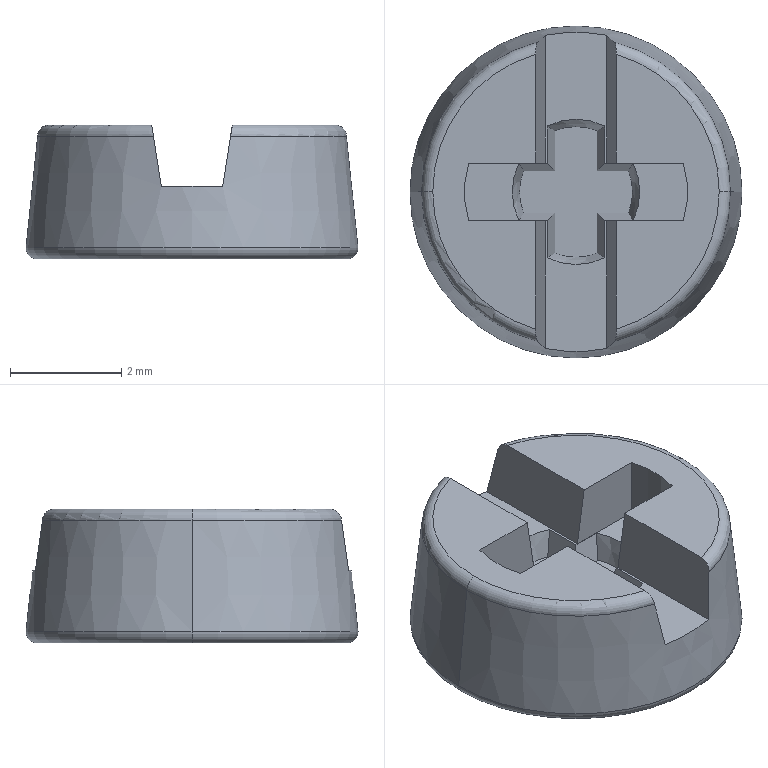Part | STEP file | 2023_07_21_12_39_19_0137 | 1 solid | 35 faces | box 5.956 x 5.956 x 2.4 mm | volume 49.622 mm3 | plane 21 | torus 6 | cone 6 | cylinder 2 | commonest cylinder face diameters 3.7 x2
STEP:
#1=CARTESIAN_POINT('',(12.522,55.,30.7));
#2=VERTEX_POINT('',#1);
#3=CARTESIAN_POINT('',(18.478,55.,30.7));
#4=VERTEX_POINT('',#3);
#5=CARTESIAN_POINT('',(15.5,55.,30.7));
#6=DIRECTION('',(0.,0.,-1.));
#7=DIRECTION('',(-1.,0.,0.));
#8=AXIS2_PLACEMENT_3D('',#5,#6,#7);
#9=CIRCLE('',#8,2.978);
#10=EDGE_CURVE('',#2,#4,#9,.T.);
#11=ORIENTED_EDGE('',*,*,#10,.T.);
#12=CARTESIAN_POINT('',(18.278,55.,30.5));
#13=VERTEX_POINT('',#12);
#14=CARTESIAN_POINT('',(18.278,55.,30.7));
#15=DIRECTION('',(0.,1.,0.));
#16=DIRECTION('',(-1.,0.,0.));
#17=AXIS2_PLACEMENT_3D('',#14,#15,#16);
#18=CIRCLE('',#17,0.2);
#19=EDGE_CURVE('',#4,#13,#18,.T.);
#20=ORIENTED_EDGE('',*,*,#19,.T.);
#21=CARTESIAN_POINT('',(12.722,55.,30.5));
#22=VERTEX_POINT('',#21);
#23=CARTESIAN_POINT('',(15.5,55.,30.5));
#24=DIRECTION('',(0.,0.,-1.));
#25=DIRECTION('',(-1.,0.,0.));
#26=AXIS2_PLACEMENT_3D('',#23,#24,#25);
#27=CIRCLE('',#26,2.778);
#28=EDGE_CURVE('',#22,#13,#27,.T.);
#29=ORIENTED_EDGE('',*,*,#28,.F.);
#30=CARTESIAN_POINT('',(12.722,55.,30.7));
#31=DIRECTION('',(0.,-1.,0.));
#32=DIRECTION('',(0.,0.,-1.));
#33=AXIS2_PLACEMENT_3D('',#30,#31,#32);
#34=CIRCLE('',#33,0.2);
#35=EDGE_CURVE('',#2,#22,#34,.T.);
#36=ORIENTED_EDGE('',*,*,#35,.F.);
#37=EDGE_LOOP('',(#11,#20,#29,#36));
#38=FACE_OUTER_BOUND('',#37,.T.);
#39=CARTESIAN_POINT('',(15.5,55.,30.7));
#40=DIRECTION('',(0.,0.,-1.));
#41=DIRECTION('',(-1.,0.,0.));
#42=AXIS2_PLACEMENT_3D('',#39,#40,#41);
#43=TOROIDAL_SURFACE('',#42,2.778,0.2);
#44=ADVANCED_FACE('',(#38),#43,.T.);
#45=CARTESIAN_POINT('',(16.192,57.682,32.7));
#46=VERTEX_POINT('',#45);
#47=CARTESIAN_POINT('',(18.27,55.,32.7));
#48=VERTEX_POINT('',#47);
#49=CARTESIAN_POINT('',(15.5,55.,32.7));
#50=DIRECTION('',(0.,0.,-1.));
#51=DIRECTION('',(-1.,0.,0.));
#52=AXIS2_PLACEMENT_3D('',#49,#50,#51);
#53=CIRCLE('',#52,2.77);
#54=EDGE_CURVE('',#46,#48,#53,.T.);
#55=ORIENTED_EDGE('',*,*,#54,.T.);
#56=CARTESIAN_POINT('',(18.374,55.,31.7));
#57=DIRECTION('',(0.1036,0.,-0.9946));
#58=VECTOR('',#57,1000.);
#59=LINE('',#56,#58);
#60=EDGE_CURVE('',#48,#4,#59,.T.);
#61=ORIENTED_EDGE('',*,*,#60,.T.);
#62=ORIENTED_EDGE('',*,*,#10,.F.);
#63=CARTESIAN_POINT('',(12.73,55.,32.7));
#64=VERTEX_POINT('',#63);
#65=CARTESIAN_POINT('',(12.626,55.,31.7));
#66=DIRECTION('',(-0.1036,0.,-0.9946));
#67=VECTOR('',#66,1000.);
#68=LINE('',#65,#67);
#69=EDGE_CURVE('',#64,#2,#68,.T.);
#70=ORIENTED_EDGE('',*,*,#69,.F.);
#71=CARTESIAN_POINT('',(14.808,57.682,32.7));
#72=VERTEX_POINT('',#71);
#73=CARTESIAN_POINT('',(15.5,55.,32.7));
#74=DIRECTION('',(0.,0.,-1.));
#75=DIRECTION('',(-1.,0.,0.));
#76=AXIS2_PLACEMENT_3D('',#73,#74,#75);
#77=CIRCLE('',#76,2.77);
#78=EDGE_CURVE('',#64,#72,#77,.T.);
#79=ORIENTED_EDGE('',*,*,#78,.T.);
#80=CARTESIAN_POINT('',(14.95,57.81,31.8));
#81=VERTEX_POINT('',#80);
#82=CARTESIAN_POINT('',(14.808,57.682,32.7));
#83=CARTESIAN_POINT('',(14.854,57.725,32.407));
#84=CARTESIAN_POINT('',(14.902,57.768,32.107));
#85=CARTESIAN_POINT('',(14.95,57.81,31.8));
#86=(BOUNDED_CURVE()B_SPLINE_CURVE(3,(#82,#83,#84,#85),.UNSPECIFIED.,.F.,.F.)B_SPLINE_CURVE_WITH_KNOTS((4,4),(3.815,3.854),.UNSPECIFIED.)CURVE()GEOMETRIC_REPRESENTATION_ITEM()RATIONAL_B_SPLINE_CURVE((1.,0.9999,0.9999,1.))REPRESENTATION_ITEM(''));
#87=EDGE_CURVE('',#72,#81,#86,.T.);
#88=ORIENTED_EDGE('',*,*,#87,.T.);
#89=CARTESIAN_POINT('',(16.05,57.81,31.8));
#90=VERTEX_POINT('',#89);
#91=CARTESIAN_POINT('',(15.5,55.,31.8));
#92=DIRECTION('',(0.,0.,-1.));
#93=DIRECTION('',(-1.,0.,0.));
#94=AXIS2_PLACEMENT_3D('',#91,#92,#93);
#95=CIRCLE('',#94,2.864);
#96=EDGE_CURVE('',#81,#90,#95,.T.);
#97=ORIENTED_EDGE('',*,*,#96,.T.);
#98=CARTESIAN_POINT('',(16.05,57.81,31.8));
#99=CARTESIAN_POINT('',(16.098,57.768,32.107));
#100=CARTESIAN_POINT('',(16.146,57.725,32.407));
#101=CARTESIAN_POINT('',(16.192,57.682,32.7));
#102=(BOUNDED_CURVE()B_SPLINE_CURVE(3,(#98,#99,#100,#101),.UNSPECIFIED.,.F.,.F.)B_SPLINE_CURVE_WITH_KNOTS((4,4),(5.571,5.61),.UNSPECIFIED.)CURVE()GEOMETRIC_REPRESENTATION_ITEM()RATIONAL_B_SPLINE_CURVE((1.,0.9999,0.9999,1.))REPRESENTATION_ITEM(''));
#103=EDGE_CURVE('',#90,#46,#102,.T.);
#104=ORIENTED_EDGE('',*,*,#103,.T.);
#105=EDGE_LOOP('',(#55,#61,#62,#70,#79,#88,#97,#104));
#106=FACE_OUTER_BOUND('',#105,.T.);
#107=CARTESIAN_POINT('',(15.5,55.,31.7));
#108=DIRECTION('',(0.,0.,-1.));
#109=DIRECTION('',(-1.,0.,0.));
#110=AXIS2_PLACEMENT_3D('',#107,#108,#109);
#111=CONICAL_SURFACE('',#110,2.874,0.1038);
#112=ADVANCED_FACE('',(#106),#111,.T.);
#113=CARTESIAN_POINT('',(14.777,52.534,32.9));
#114=VERTEX_POINT('',#113);
#115=CARTESIAN_POINT('',(12.93,55.,32.9));
#116=VERTEX_POINT('',#115);
#117=CARTESIAN_POINT('',(15.5,55.,32.9));
#118=DIRECTION('',(0.,0.,-1.));
#119=DIRECTION('',(-1.,0.,0.));
#120=AXIS2_PLACEMENT_3D('',#117,#118,#119);
#121=CIRCLE('',#120,2.57);
#122=EDGE_CURVE('',#114,#116,#121,.T.);
#123=ORIENTED_EDGE('',*,*,#122,.T.);
#124=CARTESIAN_POINT('',(12.93,55.,32.7));
#125=DIRECTION('',(0.,-1.,0.));
#126=DIRECTION('',(0.,0.,-1.));
#127=AXIS2_PLACEMENT_3D('',#124,#125,#126);
#128=CIRCLE('',#127,0.2);
#129=EDGE_CURVE('',#116,#64,#128,.T.);
#130=ORIENTED_EDGE('',*,*,#129,.T.);
#131=CARTESIAN_POINT('',(14.808,52.318,32.7));
#132=VERTEX_POINT('',#131);
#133=CARTESIAN_POINT('',(15.5,55.,32.7));
#134=DIRECTION('',(0.,0.,-1.));
#135=DIRECTION('',(-1.,0.,0.));
#136=AXIS2_PLACEMENT_3D('',#133,#134,#135);
#137=CIRCLE('',#136,2.77);
#138=EDGE_CURVE('',#132,#64,#137,.T.);
#139=ORIENTED_EDGE('',*,*,#138,.F.);
#140=CARTESIAN_POINT('',(14.808,52.318,32.7));
#141=CARTESIAN_POINT('',(14.804,52.319,32.723));
#142=CARTESIAN_POINT('',(14.8,52.324,32.748));
#143=CARTESIAN_POINT('',(14.795,52.341,32.785));
#144=CARTESIAN_POINT('',(14.793,52.347,32.797));
#145=CARTESIAN_POINT('',(14.79,52.36,32.815));
#146=CARTESIAN_POINT('',(14.789,52.367,32.823));
#147=CARTESIAN_POINT('',(14.787,52.375,32.832));
#148=CARTESIAN_POINT('',(14.787,52.38,32.837));
#149=CARTESIAN_POINT('',(14.786,52.384,32.841));
#150=CARTESIAN_POINT('',(14.784,52.4,32.855));
#151=CARTESIAN_POINT('',(14.781,52.42,32.871));
#152=CARTESIAN_POINT('',(14.777,52.489,32.898));
#153=CARTESIAN_POINT('',(14.777,52.517,32.9));
#154=CARTESIAN_POINT('',(14.777,52.534,32.9));
#155=B_SPLINE_CURVE_WITH_KNOTS('',3,(#140,#141,#142,#143,#144,#145,#146,#147,#148,#149,#150,#151,#152,#153,#154),.UNSPECIFIED.,.F.,.F.,(4,2,2,1,2,2,2,4),(0.,0.25,0.375,0.4375,0.4688,0.5,0.75,1.),.UNSPECIFIED.);
#156=EDGE_CURVE('',#132,#114,#155,.T.);
#157=ORIENTED_EDGE('',*,*,#156,.T.);
#158=EDGE_LOOP('',(#123,#130,#139,#157));
#159=FACE_OUTER_BOUND('',#158,.T.);
#160=CARTESIAN_POINT('',(15.5,55.,32.7));
#161=DIRECTION('',(0.,0.,-1.));
#162=DIRECTION('',(-1.,0.,0.));
#163=AXIS2_PLACEMENT_3D('',#160,#161,#162);
#164=TOROIDAL_SURFACE('',#163,2.57,0.2);
#165=ADVANCED_FACE('',(#159),#164,.T.);
#166=CARTESIAN_POINT('',(16.223,57.466,32.9));
#167=VERTEX_POINT('',#166);
#168=CARTESIAN_POINT('',(18.07,55.,32.9));
#169=VERTEX_POINT('',#168);
#170=CARTESIAN_POINT('',(15.5,55.,32.9));
#171=DIRECTION('',(0.,0.,-1.));
#172=DIRECTION('',(-1.,0.,0.));
#173=AXIS2_PLACEMENT_3D('',#170,#171,#172);
#174=CIRCLE('',#173,2.57);
#175=EDGE_CURVE('',#167,#169,#174,.T.);
#176=ORIENTED_EDGE('',*,*,#175,.T.);
#177=CARTESIAN_POINT('',(18.07,55.,32.7));
#178=DIRECTION('',(0.,1.,0.));
#179=DIRECTION('',(0.,0.,1.));
#180=AXIS2_PLACEMENT_3D('',#177,#178,#179);
#181=CIRCLE('',#180,0.2);
#182=EDGE_CURVE('',#169,#48,#181,.T.);
#183=ORIENTED_EDGE('',*,*,#182,.T.);
#184=ORIENTED_EDGE('',*,*,#54,.F.);
#185=CARTESIAN_POINT('',(16.192,57.682,32.7));
#186=CARTESIAN_POINT('',(16.196,57.681,32.723));
#187=CARTESIAN_POINT('',(16.2,57.676,32.748));
#188=CARTESIAN_POINT('',(16.205,57.659,32.785));
#189=CARTESIAN_POINT('',(16.207,57.653,32.797));
#190=CARTESIAN_POINT('',(16.21,57.64,32.815));
#191=CARTESIAN_POINT('',(16.211,57.633,32.823));
#192=CARTESIAN_POINT('',(16.213,57.625,32.832));
#193=CARTESIAN_POINT('',(16.213,57.62,32.837));
#194=CARTESIAN_POINT('',(16.214,57.616,32.841));
#195=CARTESIAN_POINT('',(16.216,57.6,32.855));
#196=CARTESIAN_POINT('',(16.219,57.58,32.871));
#197=CARTESIAN_POINT('',(16.223,57.511,32.898));
#198=CARTESIAN_POINT('',(16.223,57.483,32.9));
#199=CARTESIAN_POINT('',(16.223,57.466,32.9));
#200=B_SPLINE_CURVE_WITH_KNOTS('',3,(#185,#186,#187,#188,#189,#190,#191,#192,#193,#194,#195,#196,#197,#198,#199),.UNSPECIFIED.,.F.,.F.,(4,2,2,1,2,2,2,4),(0.,0.25,0.375,0.4375,0.4688,0.5,0.75,1.),.UNSPECIFIED.);
#201=EDGE_CURVE('',#46,#167,#200,.T.);
#202=ORIENTED_EDGE('',*,*,#201,.T.);
#203=EDGE_LOOP('',(#176,#183,#184,#202));
#204=FACE_OUTER_BOUND('',#203,.T.);
#205=CARTESIAN_POINT('',(15.5,55.,32.7));
#206=DIRECTION('',(0.,0.,-1.));
#207=DIRECTION('',(1.,0.,0.));
#208=AXIS2_PLACEMENT_3D('',#205,#206,#207);
#209=TOROIDAL_SURFACE('',#208,2.57,0.2);
#210=ADVANCED_FACE('',(#204),#209,.T.);
#211=ORIENTED_EDGE('',*,*,#28,.T.);
#212=CARTESIAN_POINT('',(15.5,55.,30.5));
#213=DIRECTION('',(0.,0.,-1.));
#214=DIRECTION('',(-1.,0.,0.));
#215=AXIS2_PLACEMENT_3D('',#212,#213,#214);
#216=CIRCLE('',#215,2.778);
#217=EDGE_CURVE('',#13,#22,#216,.T.);
#218=ORIENTED_EDGE('',*,*,#217,.T.);
#219=EDGE_LOOP('',(#211,#218));
#220=FACE_OUTER_BOUND('',#219,.T.);
#221=CARTESIAN_POINT('',(14.111,55.,30.5));
#222=DIRECTION('',(0.,0.,-1.));
#223=DIRECTION('',(-1.,0.,0.));
#224=AXIS2_PLACEMENT_3D('',#221,#222,#223);
#225=PLANE('',#224);
#226=ADVANCED_FACE('',(#220),#225,.T.);
#227=CARTESIAN_POINT('',(17.427,54.485,32.9));
#228=VERTEX_POINT('',#227);
#229=CARTESIAN_POINT('',(16.223,54.485,32.9));
#230=VERTEX_POINT('',#229);
#231=CARTESIAN_POINT('',(14.858,54.485,32.9));
#232=DIRECTION('',(-1.,0.,0.));
#233=VECTOR('',#232,1000.);
#234=LINE('',#231,#233);
#235=EDGE_CURVE('',#228,#230,#234,.T.);
#236=ORIENTED_EDGE('',*,*,#235,.T.);
#237=CARTESIAN_POINT('',(16.223,52.534,32.9));
#238=VERTEX_POINT('',#237);
#239=CARTESIAN_POINT('',(16.223,57.5,32.9));
#240=DIRECTION('',(0.,-1.,0.));
#241=VECTOR('',#240,1000.);
#242=LINE('',#239,#241);
#243=EDGE_CURVE('',#230,#238,#242,.T.);
#244=ORIENTED_EDGE('',*,*,#243,.T.);
#245=CARTESIAN_POINT('',(15.5,55.,32.9));
#246=DIRECTION('',(0.,0.,-1.));
#247=DIRECTION('',(-1.,0.,0.));
#248=AXIS2_PLACEMENT_3D('',#245,#246,#247);
#249=CIRCLE('',#248,2.57);
#250=EDGE_CURVE('',#169,#238,#249,.T.);
#251=ORIENTED_EDGE('',*,*,#250,.F.);
#252=ORIENTED_EDGE('',*,*,#175,.F.);
#253=CARTESIAN_POINT('',(16.223,55.515,32.9));
#254=VERTEX_POINT('',#253);
#255=CARTESIAN_POINT('',(16.223,57.5,32.9));
#256=DIRECTION('',(0.,-1.,0.));
#257=VECTOR('',#256,1000.);
#258=LINE('',#255,#257);
#259=EDGE_CURVE('',#167,#254,#258,.T.);
#260=ORIENTED_EDGE('',*,*,#259,.T.);
#261=CARTESIAN_POINT('',(17.427,55.515,32.9));
#262=VERTEX_POINT('',#261);
#263=CARTESIAN_POINT('',(14.858,55.515,32.9));
#264=DIRECTION('',(1.,0.,0.));
#265=VECTOR('',#264,1000.);
#266=LINE('',#263,#265);
#267=EDGE_CURVE('',#254,#262,#266,.T.);
#268=ORIENTED_EDGE('',*,*,#267,.T.);
#269=CARTESIAN_POINT('',(15.65,55.,32.9));
#270=DIRECTION('',(0.,0.,-1.));
#271=DIRECTION('',(0.9605,-0.2784,0.));
#272=AXIS2_PLACEMENT_3D('',#269,#270,#271);
#273=CIRCLE('',#272,1.85);
#274=EDGE_CURVE('',#262,#228,#273,.T.);
#275=ORIENTED_EDGE('',*,*,#274,.T.);
#276=EDGE_LOOP('',(#236,#244,#251,#252,#260,#268,#275));
#277=FACE_OUTER_BOUND('',#276,.T.);
#278=CARTESIAN_POINT('',(14.215,55.,32.9));
#279=DIRECTION('',(0.,0.,1.));
#280=DIRECTION('',(1.,0.,0.));
#281=AXIS2_PLACEMENT_3D('',#278,#279,#280);
#282=PLANE('',#281);
#283=ADVANCED_FACE('',(#277),#282,.T.);
#284=CARTESIAN_POINT('',(16.012,53.817,31.8));
#285=VERTEX_POINT('',#284);
#286=CARTESIAN_POINT('',(14.988,53.817,31.8));
#287=VERTEX_POINT('',#286);
#288=CARTESIAN_POINT('',(15.5,54.842,31.8));
#289=DIRECTION('',(0.,0.,-1.));
#290=DIRECTION('',(0.4485,-0.8938,0.));
#291=AXIS2_PLACEMENT_3D('',#288,#289,#290);
#292=CIRCLE('',#291,1.146);
#293=EDGE_CURVE('',#285,#287,#292,.T.);
#294=ORIENTED_EDGE('',*,*,#293,.T.);
#295=CARTESIAN_POINT('',(14.988,54.488,31.8));
#296=VERTEX_POINT('',#295);
#297=CARTESIAN_POINT('',(14.988,57.243,31.8));
#298=DIRECTION('',(0.,1.,0.));
#299=VECTOR('',#298,1000.);
#300=LINE('',#297,#299);
#301=EDGE_CURVE('',#287,#296,#300,.T.);
#302=ORIENTED_EDGE('',*,*,#301,.T.);
#303=CARTESIAN_POINT('',(14.475,54.488,31.8));
#304=VERTEX_POINT('',#303);
#305=CARTESIAN_POINT('',(14.987,54.488,31.8));
#306=DIRECTION('',(-1.,0.,0.));
#307=VECTOR('',#306,1000.);
#308=LINE('',#305,#307);
#309=EDGE_CURVE('',#296,#304,#308,.T.);
#310=ORIENTED_EDGE('',*,*,#309,.T.);
#311=CARTESIAN_POINT('',(14.475,55.512,31.8));
#312=VERTEX_POINT('',#311);
#313=CARTESIAN_POINT('',(15.5,55.,31.8));
#314=DIRECTION('',(0.,0.,-1.));
#315=DIRECTION('',(-0.8938,-0.4485,0.));
#316=AXIS2_PLACEMENT_3D('',#313,#314,#315);
#317=CIRCLE('',#316,1.146);
#318=EDGE_CURVE('',#304,#312,#317,.T.);
#319=ORIENTED_EDGE('',*,*,#318,.T.);
#320=CARTESIAN_POINT('',(14.988,55.512,31.8));
#321=VERTEX_POINT('',#320);
#322=CARTESIAN_POINT('',(15.243,55.512,31.8));
#323=DIRECTION('',(1.,0.,0.));
#324=VECTOR('',#323,1000.);
#325=LINE('',#322,#324);
#326=EDGE_CURVE('',#312,#321,#325,.T.);
#327=ORIENTED_EDGE('',*,*,#326,.T.);
#328=CARTESIAN_POINT('',(14.988,56.183,31.8));
#329=VERTEX_POINT('',#328);
#330=CARTESIAN_POINT('',(14.988,58.092,31.8));
#331=DIRECTION('',(0.,1.,0.));
#332=VECTOR('',#331,1000.);
#333=LINE('',#330,#332);
#334=EDGE_CURVE('',#321,#329,#333,.T.);
#335=ORIENTED_EDGE('',*,*,#334,.T.);
#336=CARTESIAN_POINT('',(16.012,56.183,31.8));
#337=VERTEX_POINT('',#336);
#338=CARTESIAN_POINT('',(15.5,55.158,31.8));
#339=DIRECTION('',(0.,0.,-1.));
#340=DIRECTION('',(-0.4485,0.8938,0.));
#341=AXIS2_PLACEMENT_3D('',#338,#339,#340);
#342=CIRCLE('',#341,1.146);
#343=EDGE_CURVE('',#329,#337,#342,.T.);
#344=ORIENTED_EDGE('',*,*,#343,.T.);
#345=CARTESIAN_POINT('',(16.012,55.512,31.8));
#346=VERTEX_POINT('',#345);
#347=CARTESIAN_POINT('',(16.012,57.758,31.8));
#348=DIRECTION('',(0.,-1.,0.));
#349=VECTOR('',#348,1000.);
#350=LINE('',#347,#349);
#351=EDGE_CURVE('',#337,#346,#350,.T.);
#352=ORIENTED_EDGE('',*,*,#351,.T.);
#353=CARTESIAN_POINT('',(16.525,55.512,31.8));
#354=VERTEX_POINT('',#353);
#355=CARTESIAN_POINT('',(16.013,55.512,31.8));
#356=DIRECTION('',(1.,0.,0.));
#357=VECTOR('',#356,1000.);
#358=LINE('',#355,#357);
#359=EDGE_CURVE('',#346,#354,#358,.T.);
#360=ORIENTED_EDGE('',*,*,#359,.T.);
#361=CARTESIAN_POINT('',(16.525,54.488,31.8));
#362=VERTEX_POINT('',#361);
#363=CARTESIAN_POINT('',(15.5,55.,31.8));
#364=DIRECTION('',(0.,0.,-1.));
#365=DIRECTION('',(0.8938,0.4485,0.));
#366=AXIS2_PLACEMENT_3D('',#363,#364,#365);
#367=CIRCLE('',#366,1.146);
#368=EDGE_CURVE('',#354,#362,#367,.T.);
#369=ORIENTED_EDGE('',*,*,#368,.T.);
#370=CARTESIAN_POINT('',(16.012,54.488,31.8));
#371=VERTEX_POINT('',#370);
#372=CARTESIAN_POINT('',(15.758,54.488,31.8));
#373=DIRECTION('',(-1.,0.,0.));
#374=VECTOR('',#373,1000.);
#375=LINE('',#372,#374);
#376=EDGE_CURVE('',#362,#371,#375,.T.);
#377=ORIENTED_EDGE('',*,*,#376,.T.);
#378=CARTESIAN_POINT('',(16.012,56.908,31.8));
#379=DIRECTION('',(0.,-1.,0.));
#380=VECTOR('',#379,1000.);
#381=LINE('',#378,#380);
#382=EDGE_CURVE('',#371,#285,#381,.T.);
#383=ORIENTED_EDGE('',*,*,#382,.T.);
#384=EDGE_LOOP('',(#294,#302,#310,#319,#327,#335,#344,#352,#360,#369,#377,#383));
#385=FACE_BOUND('',#384,.T.);
#386=CARTESIAN_POINT('',(16.05,54.485,31.8));
#387=VERTEX_POINT('',#386);
#388=CARTESIAN_POINT('',(16.05,52.19,31.8));
#389=VERTEX_POINT('',#388);
#390=CARTESIAN_POINT('',(16.05,60.,31.8));
#391=DIRECTION('',(0.,-1.,0.));
#392=VECTOR('',#391,1000.);
#393=LINE('',#390,#392);
#394=EDGE_CURVE('',#387,#389,#393,.T.);
#395=ORIENTED_EDGE('',*,*,#394,.F.);
#396=CARTESIAN_POINT('',(17.427,54.485,31.8));
#397=VERTEX_POINT('',#396);
#398=CARTESIAN_POINT('',(13.573,54.485,31.8));
#399=DIRECTION('',(1.,0.,0.));
#400=VECTOR('',#399,1000.);
#401=LINE('',#398,#400);
#402=EDGE_CURVE('',#387,#397,#401,.T.);
#403=ORIENTED_EDGE('',*,*,#402,.T.);
#404=CARTESIAN_POINT('',(17.427,55.515,31.8));
#405=VERTEX_POINT('',#404);
#406=CARTESIAN_POINT('',(15.65,55.,31.8));
#407=DIRECTION('',(0.,0.,1.));
#408=DIRECTION('',(0.9605,-0.2784,0.));
#409=AXIS2_PLACEMENT_3D('',#406,#407,#408);
#410=CIRCLE('',#409,1.85);
#411=EDGE_CURVE('',#397,#405,#410,.T.);
#412=ORIENTED_EDGE('',*,*,#411,.T.);
#413=CARTESIAN_POINT('',(16.05,55.515,31.8));
#414=VERTEX_POINT('',#413);
#415=CARTESIAN_POINT('',(17.427,55.515,31.8));
#416=DIRECTION('',(-1.,0.,0.));
#417=VECTOR('',#416,1000.);
#418=LINE('',#415,#417);
#419=EDGE_CURVE('',#405,#414,#418,.T.);
#420=ORIENTED_EDGE('',*,*,#419,.T.);
#421=CARTESIAN_POINT('',(16.05,60.,31.8));
#422=DIRECTION('',(0.,-1.,0.));
#423=VECTOR('',#422,1000.);
#424=LINE('',#421,#423);
#425=EDGE_CURVE('',#90,#414,#424,.T.);
#426=ORIENTED_EDGE('',*,*,#425,.F.);
#427=ORIENTED_EDGE('',*,*,#96,.F.);
#428=CARTESIAN_POINT('',(14.95,55.515,31.8));
#429=VERTEX_POINT('',#428);
#430=CARTESIAN_POINT('',(14.95,60.,31.8));
#431=DIRECTION('',(0.,-1.,0.));
#432=VECTOR('',#431,1000.);
#433=LINE('',#430,#432);
#434=EDGE_CURVE('',#81,#429,#433,.T.);
#435=ORIENTED_EDGE('',*,*,#434,.T.);
#436=CARTESIAN_POINT('',(13.573,55.515,31.8));
#437=VERTEX_POINT('',#436);
#438=CARTESIAN_POINT('',(17.427,55.515,31.8));
#439=DIRECTION('',(-1.,0.,0.));
#440=VECTOR('',#439,1000.);
#441=LINE('',#438,#440);
#442=EDGE_CURVE('',#429,#437,#441,.T.);
#443=ORIENTED_EDGE('',*,*,#442,.T.);
#444=CARTESIAN_POINT('',(13.573,54.485,31.8));
#445=VERTEX_POINT('',#444);
#446=CARTESIAN_POINT('',(15.35,55.,31.8));
#447=DIRECTION('',(0.,0.,1.));
#448=DIRECTION('',(-0.9605,0.2784,0.));
#449=AXIS2_PLACEMENT_3D('',#446,#447,#448);
#450=CIRCLE('',#449,1.85);
#451=EDGE_CURVE('',#437,#445,#450,.T.);
#452=ORIENTED_EDGE('',*,*,#451,.T.);
#453=CARTESIAN_POINT('',(14.95,54.485,31.8));
#454=VERTEX_POINT('',#453);
#455=CARTESIAN_POINT('',(13.573,54.485,31.8));
#456=DIRECTION('',(1.,0.,0.));
#457=VECTOR('',#456,1000.);
#458=LINE('',#455,#457);
#459=EDGE_CURVE('',#445,#454,#458,.T.);
#460=ORIENTED_EDGE('',*,*,#459,.T.);
#461=CARTESIAN_POINT('',(14.95,52.19,31.8));
#462=VERTEX_POINT('',#461);
#463=CARTESIAN_POINT('',(14.95,60.,31.8));
#464=DIRECTION('',(0.,-1.,0.));
#465=VECTOR('',#464,1000.);
#466=LINE('',#463,#465);
#467=EDGE_CURVE('',#454,#462,#466,.T.);
#468=ORIENTED_EDGE('',*,*,#467,.T.);
#469=CARTESIAN_POINT('',(15.5,55.,31.8));
#470=DIRECTION('',(0.,0.,-1.));
#471=DIRECTION('',(-1.,0.,0.));
#472=AXIS2_PLACEMENT_3D('',#469,#470,#471);
#473=CIRCLE('',#472,2.864);
#474=EDGE_CURVE('',#389,#462,#473,.T.);
#475=ORIENTED_EDGE('',*,*,#474,.F.);
#476=EDGE_LOOP('',(#395,#403,#412,#420,#426,#427,#435,#443,#452,#460,#468,#475));
#477=FACE_OUTER_BOUND('',#476,.T.);
#478=CARTESIAN_POINT('',(15.5,60.,31.8));
#479=DIRECTION('',(0.,0.,-1.));
#480=DIRECTION('',(0.,-1.,0.));
#481=AXIS2_PLACEMENT_3D('',#478,#479,#480);
#482=PLANE('',#481);
#483=ADVANCED_FACE('',(#385,#477),#482,.F.);
#484=CARTESIAN_POINT('',(14.777,54.485,32.9));
#485=VERTEX_POINT('',#484);
#486=CARTESIAN_POINT('',(14.913,54.485,32.033));
#487=DIRECTION('',(-0.1557,0.,0.9878));
#488=VECTOR('',#487,1000.);
#489=LINE('',#486,#488);
#490=EDGE_CURVE('',#454,#485,#489,.T.);
#491=ORIENTED_EDGE('',*,*,#490,.T.);
#492=CARTESIAN_POINT('',(14.777,57.5,32.9));
#493=DIRECTION('',(0.,1.,0.));
#494=VECTOR('',#493,1000.);
#495=LINE('',#492,#494);
#496=EDGE_CURVE('',#114,#485,#495,.T.);
#497=ORIENTED_EDGE('',*,*,#496,.F.);
#498=ORIENTED_EDGE('',*,*,#156,.F.);
#499=CARTESIAN_POINT('',(14.95,52.19,31.8));
#500=CARTESIAN_POINT('',(14.902,52.232,32.107));
#501=CARTESIAN_POINT('',(14.854,52.275,32.407));
#502=CARTESIAN_POINT('',(14.808,52.318,32.7));
#503=(BOUNDED_CURVE()B_SPLINE_CURVE(3,(#499,#500,#501,#502),.UNSPECIFIED.,.F.,.F.)B_SPLINE_CURVE_WITH_KNOTS((4,4),(2.429,2.468),.UNSPECIFIED.)CURVE()GEOMETRIC_REPRESENTATION_ITEM()RATIONAL_B_SPLINE_CURVE((1.,0.9999,0.9999,1.))REPRESENTATION_ITEM(''));
#504=EDGE_CURVE('',#462,#132,#503,.T.);
#505=ORIENTED_EDGE('',*,*,#504,.F.);
#506=ORIENTED_EDGE('',*,*,#467,.F.);
#507=EDGE_LOOP('',(#491,#497,#498,#505,#506));
#508=FACE_OUTER_BOUND('',#507,.T.);
#509=CARTESIAN_POINT('',(14.863,60.,32.35));
#510=DIRECTION('',(-0.9878,0.,-0.1557));
#511=DIRECTION('',(-0.1557,0.,0.9878));
#512=AXIS2_PLACEMENT_3D('',#509,#510,#511);
#513=PLANE('',#512);
#514=ADVANCED_FACE('',(#508),#513,.F.);
#515=CARTESIAN_POINT('',(16.087,54.485,32.033));
#516=DIRECTION('',(-0.1557,0.,-0.9878));
#517=VECTOR('',#516,1000.);
#518=LINE('',#515,#517);
#519=EDGE_CURVE('',#230,#387,#518,.T.);
#520=ORIENTED_EDGE('',*,*,#519,.T.);
#521=ORIENTED_EDGE('',*,*,#394,.T.);
#522=CARTESIAN_POINT('',(16.192,52.318,32.7));
#523=VERTEX_POINT('',#522);
#524=CARTESIAN_POINT('',(16.192,52.318,32.7));
#525=CARTESIAN_POINT('',(16.146,52.275,32.407));
#526=CARTESIAN_POINT('',(16.098,52.232,32.107));
#527=CARTESIAN_POINT('',(16.05,52.19,31.8));
#528=(BOUNDED_CURVE()B_SPLINE_CURVE(3,(#524,#525,#526,#527),.UNSPECIFIED.,.F.,.F.)B_SPLINE_CURVE_WITH_KNOTS((4,4),(0.6735,0.7123),.UNSPECIFIED.)CURVE()GEOMETRIC_REPRESENTATION_ITEM()RATIONAL_B_SPLINE_CURVE((1.,0.9999,0.9999,1.))REPRESENTATION_ITEM(''));
#529=EDGE_CURVE('',#523,#389,#528,.T.);
#530=ORIENTED_EDGE('',*,*,#529,.F.);
#531=CARTESIAN_POINT('',(16.223,52.534,32.9));
#532=CARTESIAN_POINT('',(16.223,52.517,32.9));
#533=CARTESIAN_POINT('',(16.223,52.487,32.898));
#534=CARTESIAN_POINT('',(16.22,52.438,32.879));
#535=CARTESIAN_POINT('',(16.219,52.424,32.871));
#536=CARTESIAN_POINT('',(16.217,52.407,32.86));
#537=CARTESIAN_POINT('',(16.217,52.402,32.856));
#538=CARTESIAN_POINT('',(16.216,52.395,32.851));
#539=CARTESIAN_POINT('',(16.215,52.393,32.849));
#540=CARTESIAN_POINT('',(16.215,52.389,32.846));
#541=CARTESIAN_POINT('',(16.215,52.388,32.845));
#542=CARTESIAN_POINT('',(16.208,52.34,32.801));
#543=CARTESIAN_POINT('',(16.199,52.32,32.746));
#544=CARTESIAN_POINT('',(16.192,52.318,32.7));
#545=B_SPLINE_CURVE_WITH_KNOTS('',3,(#531,#532,#533,#534,#535,#536,#537,#538,#539,#540,#541,#542,#543,#544),.UNSPECIFIED.,.F.,.F.,(4,2,2,2,2,2,4),(0.,0.25,0.375,0.4375,0.4687,0.5,1.),.UNSPECIFIED.);
#546=EDGE_CURVE('',#238,#523,#545,.T.);
#547=ORIENTED_EDGE('',*,*,#546,.F.);
#548=ORIENTED_EDGE('',*,*,#243,.F.);
#549=EDGE_LOOP('',(#520,#521,#530,#547,#548));
#550=FACE_OUTER_BOUND('',#549,.T.);
#551=CARTESIAN_POINT('',(16.137,60.,32.35));
#552=DIRECTION('',(0.9878,0.,-0.1557));
#553=DIRECTION('',(0.,-1.,0.));
#554=AXIS2_PLACEMENT_3D('',#551,#552,#553);
#555=PLANE('',#554);
#556=ADVANCED_FACE('',(#550),#555,.F.);
#557=CARTESIAN_POINT('',(16.087,55.515,32.033));
#558=DIRECTION('',(0.1557,0.,0.9878));
#559=VECTOR('',#558,1000.);
#560=LINE('',#557,#559);
#561=EDGE_CURVE('',#414,#254,#560,.T.);
#562=ORIENTED_EDGE('',*,*,#561,.T.);
#563=ORIENTED_EDGE('',*,*,#259,.F.);
#564=ORIENTED_EDGE('',*,*,#201,.F.);
#565=ORIENTED_EDGE('',*,*,#103,.F.);
#566=ORIENTED_EDGE('',*,*,#425,.T.);
#567=EDGE_LOOP('',(#562,#563,#564,#565,#566));
#568=FACE_OUTER_BOUND('',#567,.T.);
#569=CARTESIAN_POINT('',(16.137,60.,32.35));
#570=DIRECTION('',(0.9878,0.,-0.1557));
#571=DIRECTION('',(0.,-1.,0.));
#572=AXIS2_PLACEMENT_3D('',#569,#570,#571);
#573=PLANE('',#572);
#574=ADVANCED_FACE('',(#568),#573,.F.);
#575=CARTESIAN_POINT('',(14.777,55.515,32.9));
#576=VERTEX_POINT('',#575);
#577=CARTESIAN_POINT('',(14.913,55.515,32.033));
#578=DIRECTION('',(0.1557,0.,-0.9878));
#579=VECTOR('',#578,1000.);
#580=LINE('',#577,#579);
#581=EDGE_CURVE('',#576,#429,#580,.T.);
#582=ORIENTED_EDGE('',*,*,#581,.T.);
#583=ORIENTED_EDGE('',*,*,#434,.F.);
#584=ORIENTED_EDGE('',*,*,#87,.F.);
#585=CARTESIAN_POINT('',(14.777,57.466,32.9));
#586=VERTEX_POINT('',#585);
#587=CARTESIAN_POINT('',(14.777,57.466,32.9));
#588=CARTESIAN_POINT('',(14.777,57.483,32.9));
#589=CARTESIAN_POINT('',(14.777,57.513,32.898));
#590=CARTESIAN_POINT('',(14.78,57.562,32.879));
#591=CARTESIAN_POINT('',(14.781,57.576,32.871));
#592=CARTESIAN_POINT('',(14.783,57.593,32.86));
#593=CARTESIAN_POINT('',(14.783,57.598,32.856));
#594=CARTESIAN_POINT('',(14.784,57.605,32.851));
#595=CARTESIAN_POINT('',(14.785,57.607,32.849));
#596=CARTESIAN_POINT('',(14.785,57.611,32.846));
#597=CARTESIAN_POINT('',(14.785,57.612,32.845));
#598=CARTESIAN_POINT('',(14.792,57.66,32.801));
#599=CARTESIAN_POINT('',(14.801,57.68,32.746));
#600=CARTESIAN_POINT('',(14.808,57.682,32.7));
#601=B_SPLINE_CURVE_WITH_KNOTS('',3,(#587,#588,#589,#590,#591,#592,#593,#594,#595,#596,#597,#598,#599,#600),.UNSPECIFIED.,.F.,.F.,(4,2,2,2,2,2,4),(0.,0.25,0.375,0.4375,0.4688,0.5,1.),.UNSPECIFIED.);
#602=EDGE_CURVE('',#586,#72,#601,.T.);
#603=ORIENTED_EDGE('',*,*,#602,.F.);
#604=CARTESIAN_POINT('',(14.777,57.5,32.9));
#605=DIRECTION('',(0.,1.,0.));
#606=VECTOR('',#605,1000.);
#607=LINE('',#604,#606);
#608=EDGE_CURVE('',#576,#586,#607,.T.);
#609=ORIENTED_EDGE('',*,*,#608,.F.);
#610=EDGE_LOOP('',(#582,#583,#584,#603,#609));
#611=FACE_OUTER_BOUND('',#610,.T.);
#612=CARTESIAN_POINT('',(14.863,60.,32.35));
#613=DIRECTION('',(-0.9878,0.,-0.1557));
#614=DIRECTION('',(-0.1557,0.,0.9878));
#615=AXIS2_PLACEMENT_3D('',#612,#613,#614);
#616=PLANE('',#615);
#617=ADVANCED_FACE('',(#611),#616,.F.);
#618=CARTESIAN_POINT('',(13.573,54.485,32.9));
#619=VERTEX_POINT('',#618);
#620=CARTESIAN_POINT('',(14.858,54.485,32.9));
#621=DIRECTION('',(-1.,0.,0.));
#622=VECTOR('',#621,1000.);
#623=LINE('',#620,#622);
#624=EDGE_CURVE('',#485,#619,#623,.T.);
#625=ORIENTED_EDGE('',*,*,#624,.T.);
#626=CARTESIAN_POINT('',(13.573,55.515,32.9));
#627=VERTEX_POINT('',#626);
#628=CARTESIAN_POINT('',(15.35,55.,32.9));
#629=DIRECTION('',(0.,0.,-1.));
#630=DIRECTION('',(-0.9605,0.2784,0.));
#631=AXIS2_PLACEMENT_3D('',#628,#629,#630);
#632=CIRCLE('',#631,1.85);
#633=EDGE_CURVE('',#619,#627,#632,.T.);
#634=ORIENTED_EDGE('',*,*,#633,.T.);
#635=CARTESIAN_POINT('',(14.858,55.515,32.9));
#636=DIRECTION('',(1.,0.,0.));
#637=VECTOR('',#636,1000.);
#638=LINE('',#635,#637);
#639=EDGE_CURVE('',#627,#576,#638,.T.);
#640=ORIENTED_EDGE('',*,*,#639,.T.);
#641=ORIENTED_EDGE('',*,*,#608,.T.);
#642=CARTESIAN_POINT('',(15.5,55.,32.9));
#643=DIRECTION('',(0.,0.,-1.));
#644=DIRECTION('',(-1.,0.,0.));
#645=AXIS2_PLACEMENT_3D('',#642,#643,#644);
#646=CIRCLE('',#645,2.57);
#647=EDGE_CURVE('',#116,#586,#646,.T.);
#648=ORIENTED_EDGE('',*,*,#647,.F.);
#649=ORIENTED_EDGE('',*,*,#122,.F.);
#650=ORIENTED_EDGE('',*,*,#496,.T.);
#651=EDGE_LOOP('',(#625,#634,#640,#641,#648,#649,#650));
#652=FACE_OUTER_BOUND('',#651,.T.);
#653=CARTESIAN_POINT('',(14.215,55.,32.9));
#654=DIRECTION('',(0.,0.,1.));
#655=DIRECTION('',(1.,0.,0.));
#656=AXIS2_PLACEMENT_3D('',#653,#654,#655);
#657=PLANE('',#656);
#658=ADVANCED_FACE('',(#652),#657,.T.);
#659=ORIENTED_EDGE('',*,*,#624,.F.);
#660=ORIENTED_EDGE('',*,*,#490,.F.);
#661=ORIENTED_EDGE('',*,*,#459,.F.);
#662=CARTESIAN_POINT('',(13.573,54.485,31.8));
#663=DIRECTION('',(0.,0.,1.));
#664=VECTOR('',#663,1000.);
#665=LINE('',#662,#664);
#666=EDGE_CURVE('',#445,#619,#665,.T.);
#667=ORIENTED_EDGE('',*,*,#666,.T.);
#668=EDGE_LOOP('',(#659,#660,#661,#667));
#669=FACE_OUTER_BOUND('',#668,.T.);
#670=CARTESIAN_POINT('',(15.5,54.485,31.8));
#671=DIRECTION('',(0.,-1.,0.));
#672=DIRECTION('',(0.,0.,-1.));
#673=AXIS2_PLACEMENT_3D('',#670,#671,#672);
#674=PLANE('',#673);
#675=ADVANCED_FACE('',(#669),#674,.F.);
#676=ORIENTED_EDGE('',*,*,#274,.F.);
#677=CARTESIAN_POINT('',(17.427,55.515,31.8));
#678=DIRECTION('',(0.,0.,1.));
#679=VECTOR('',#678,1000.);
#680=LINE('',#677,#679);
#681=EDGE_CURVE('',#405,#262,#680,.T.);
#682=ORIENTED_EDGE('',*,*,#681,.F.);
#683=ORIENTED_EDGE('',*,*,#411,.F.);
#684=CARTESIAN_POINT('',(17.427,54.485,31.8));
#685=DIRECTION('',(0.,0.,1.));
#686=VECTOR('',#685,1000.);
#687=LINE('',#684,#686);
#688=EDGE_CURVE('',#397,#228,#687,.T.);
#689=ORIENTED_EDGE('',*,*,#688,.T.);
#690=EDGE_LOOP('',(#676,#682,#683,#689));
#691=FACE_OUTER_BOUND('',#690,.T.);
#692=CARTESIAN_POINT('',(15.65,55.,31.8));
#693=DIRECTION('',(0.,0.,-1.));
#694=DIRECTION('',(0.9605,-0.2784,0.));
#695=AXIS2_PLACEMENT_3D('',#692,#693,#694);
#696=CYLINDRICAL_SURFACE('',#695,1.85);
#697=ADVANCED_FACE('',(#691),#696,.F.);
#698=ORIENTED_EDGE('',*,*,#639,.F.);
#699=CARTESIAN_POINT('',(13.573,55.515,31.8));
#700=DIRECTION('',(0.,0.,1.));
#701=VECTOR('',#700,1000.);
#702=LINE('',#699,#701);
#703=EDGE_CURVE('',#437,#627,#702,.T.);
#704=ORIENTED_EDGE('',*,*,#703,.F.);
#705=ORIENTED_EDGE('',*,*,#442,.F.);
#706=ORIENTED_EDGE('',*,*,#581,.F.);
#707=EDGE_LOOP('',(#698,#704,#705,#706));
#708=FACE_OUTER_BOUND('',#707,.T.);
#709=CARTESIAN_POINT('',(15.5,55.515,31.8));
#710=DIRECTION('',(0.,1.,0.));
#711=DIRECTION('',(1.,0.,0.));
#712=AXIS2_PLACEMENT_3D('',#709,#710,#711);
#713=PLANE('',#712);
#714=ADVANCED_FACE('',(#708),#713,.F.);
#715=ORIENTED_EDGE('',*,*,#267,.F.);
#716=ORIENTED_EDGE('',*,*,#561,.F.);
#717=ORIENTED_EDGE('',*,*,#419,.F.);
#718=ORIENTED_EDGE('',*,*,#681,.T.);
#719=EDGE_LOOP('',(#715,#716,#717,#718));
#720=FACE_OUTER_BOUND('',#719,.T.);
#721=CARTESIAN_POINT('',(15.5,55.515,31.8));
#722=DIRECTION('',(0.,1.,0.));
#723=DIRECTION('',(1.,0.,0.));
#724=AXIS2_PLACEMENT_3D('',#721,#722,#723);
#725=PLANE('',#724);
#726=ADVANCED_FACE('',(#720),#725,.F.);
#727=ORIENTED_EDGE('',*,*,#235,.F.);
#728=ORIENTED_EDGE('',*,*,#688,.F.);
#729=ORIENTED_EDGE('',*,*,#402,.F.);
#730=ORIENTED_EDGE('',*,*,#519,.F.);
#731=EDGE_LOOP('',(#727,#728,#729,#730));
#732=FACE_OUTER_BOUND('',#731,.T.);
#733=CARTESIAN_POINT('',(15.5,54.485,31.8));
#734=DIRECTION('',(0.,-1.,0.));
#735=DIRECTION('',(0.,0.,-1.));
#736=AXIS2_PLACEMENT_3D('',#733,#734,#735);
#737=PLANE('',#736);
#738=ADVANCED_FACE('',(#732),#737,.F.);
#739=ORIENTED_EDGE('',*,*,#633,.F.);
#740=ORIENTED_EDGE('',*,*,#666,.F.);
#741=ORIENTED_EDGE('',*,*,#451,.F.);
#742=ORIENTED_EDGE('',*,*,#703,.T.);
#743=EDGE_LOOP('',(#739,#740,#741,#742));
#744=FACE_OUTER_BOUND('',#743,.T.);
#745=CARTESIAN_POINT('',(15.35,55.,31.8));
#746=DIRECTION('',(0.,0.,-1.));
#747=DIRECTION('',(-0.9605,0.2784,0.));
#748=AXIS2_PLACEMENT_3D('',#745,#746,#747);
#749=CYLINDRICAL_SURFACE('',#748,1.85);
#750=ADVANCED_FACE('',(#744),#749,.F.);
#751=CARTESIAN_POINT('',(15.119,53.902,31.31));
#752=VERTEX_POINT('',#751);
#753=CARTESIAN_POINT('',(15.881,53.902,31.31));
#754=VERTEX_POINT('',#753);
#755=CARTESIAN_POINT('',(15.5,54.842,31.31));
#756=DIRECTION('',(0.,0.,1.));
#757=DIRECTION('',(0.4485,-0.8938,0.));
#758=AXIS2_PLACEMENT_3D('',#755,#756,#757);
#759=CIRCLE('',#758,1.014);
#760=EDGE_CURVE('',#752,#754,#759,.T.);
#761=ORIENTED_EDGE('',*,*,#760,.T.);
#762=CARTESIAN_POINT('',(15.881,54.619,31.31));
#763=VERTEX_POINT('',#762);
#764=CARTESIAN_POINT('',(15.881,53.816,31.31));
#765=DIRECTION('',(0.,1.,0.));
#766=VECTOR('',#765,1000.);
#767=LINE('',#764,#766);
#768=EDGE_CURVE('',#754,#763,#767,.T.);
#769=ORIENTED_EDGE('',*,*,#768,.T.);
#770=CARTESIAN_POINT('',(16.44,54.619,31.31));
#771=VERTEX_POINT('',#770);
#772=CARTESIAN_POINT('',(16.015,54.619,31.31));
#773=DIRECTION('',(1.,0.,0.));
#774=VECTOR('',#773,1000.);
#775=LINE('',#772,#774);
#776=EDGE_CURVE('',#763,#771,#775,.T.);
#777=ORIENTED_EDGE('',*,*,#776,.T.);
#778=CARTESIAN_POINT('',(16.44,55.381,31.31));
#779=VERTEX_POINT('',#778);
#780=CARTESIAN_POINT('',(15.5,55.,31.31));
#781=DIRECTION('',(0.,0.,1.));
#782=DIRECTION('',(0.8938,0.4485,0.));
#783=AXIS2_PLACEMENT_3D('',#780,#781,#782);
#784=CIRCLE('',#783,1.014);
#785=EDGE_CURVE('',#771,#779,#784,.T.);
#786=ORIENTED_EDGE('',*,*,#785,.T.);
#787=CARTESIAN_POINT('',(15.881,55.381,31.31));
#788=VERTEX_POINT('',#787);
#789=CARTESIAN_POINT('',(16.526,55.381,31.31));
#790=DIRECTION('',(-1.,0.,0.));
#791=VECTOR('',#790,1000.);
#792=LINE('',#789,#791);
#793=EDGE_CURVE('',#779,#788,#792,.T.);
#794=ORIENTED_EDGE('',*,*,#793,.T.);
#795=CARTESIAN_POINT('',(15.881,56.098,31.31));
#796=VERTEX_POINT('',#795);
#797=CARTESIAN_POINT('',(15.881,55.515,31.31));
#798=DIRECTION('',(0.,1.,0.));
#799=VECTOR('',#798,1000.);
#800=LINE('',#797,#799);
#801=EDGE_CURVE('',#788,#796,#800,.T.);
#802=ORIENTED_EDGE('',*,*,#801,.T.);
#803=CARTESIAN_POINT('',(15.119,56.098,31.31));
#804=VERTEX_POINT('',#803);
#805=CARTESIAN_POINT('',(15.5,55.158,31.31));
#806=DIRECTION('',(0.,0.,1.));
#807=DIRECTION('',(-0.4485,0.8938,0.));
#808=AXIS2_PLACEMENT_3D('',#805,#806,#807);
#809=CIRCLE('',#808,1.014);
#810=EDGE_CURVE('',#796,#804,#809,.T.);
#811=ORIENTED_EDGE('',*,*,#810,.T.);
#812=CARTESIAN_POINT('',(15.119,55.381,31.31));
#813=VERTEX_POINT('',#812);
#814=CARTESIAN_POINT('',(15.119,56.184,31.31));
#815=DIRECTION('',(0.,-1.,0.));
#816=VECTOR('',#815,1000.);
#817=LINE('',#814,#816);
#818=EDGE_CURVE('',#804,#813,#817,.T.);
#819=ORIENTED_EDGE('',*,*,#818,.T.);
#820=CARTESIAN_POINT('',(14.56,55.381,31.31));
#821=VERTEX_POINT('',#820);
#822=CARTESIAN_POINT('',(14.985,55.381,31.31));
#823=DIRECTION('',(-1.,0.,0.));
#824=VECTOR('',#823,1000.);
#825=LINE('',#822,#824);
#826=EDGE_CURVE('',#813,#821,#825,.T.);
#827=ORIENTED_EDGE('',*,*,#826,.T.);
#828=CARTESIAN_POINT('',(14.56,54.619,31.31));
#829=VERTEX_POINT('',#828);
#830=CARTESIAN_POINT('',(15.5,55.,31.31));
#831=DIRECTION('',(0.,0.,1.));
#832=DIRECTION('',(-0.8938,-0.4485,0.));
#833=AXIS2_PLACEMENT_3D('',#830,#831,#832);
#834=CIRCLE('',#833,1.014);
#835=EDGE_CURVE('',#821,#829,#834,.T.);
#836=ORIENTED_EDGE('',*,*,#835,.T.);
#837=CARTESIAN_POINT('',(15.119,54.619,31.31));
#838=VERTEX_POINT('',#837);
#839=CARTESIAN_POINT('',(14.474,54.619,31.31));
#840=DIRECTION('',(1.,0.,0.));
#841=VECTOR('',#840,1000.);
#842=LINE('',#839,#841);
#843=EDGE_CURVE('',#829,#838,#842,.T.);
#844=ORIENTED_EDGE('',*,*,#843,.T.);
#845=CARTESIAN_POINT('',(15.119,54.485,31.31));
#846=DIRECTION('',(0.,-1.,0.));
#847=VECTOR('',#846,1000.);
#848=LINE('',#845,#847);
#849=EDGE_CURVE('',#838,#752,#848,.T.);
#850=ORIENTED_EDGE('',*,*,#849,.T.);
#851=EDGE_LOOP('',(#761,#769,#777,#786,#794,#802,#811,#819,#827,#836,#844,#850));
#852=FACE_OUTER_BOUND('',#851,.T.);
#853=CARTESIAN_POINT('',(15.5,55.,31.31));
#854=DIRECTION('',(0.,0.,-1.));
#855=DIRECTION('',(0.,-1.,0.));
#856=AXIS2_PLACEMENT_3D('',#853,#854,#855);
#857=PLANE('',#856);
#858=ADVANCED_FACE('',(#852),#857,.F.);
#859=ORIENTED_EDGE('',*,*,#301,.F.);
#860=CARTESIAN_POINT('',(14.988,53.817,31.8));
#861=CARTESIAN_POINT('',(15.056,53.86,31.544));
#862=CARTESIAN_POINT('',(15.119,53.902,31.31));
#863=B_SPLINE_CURVE_WITH_KNOTS('',2,(#860,#861,#862),.UNSPECIFIED.,.F.,.F.,(3,3),(0.06011,0.5746),.UNSPECIFIED.);
#864=EDGE_CURVE('',#287,#752,#863,.T.);
#865=ORIENTED_EDGE('',*,*,#864,.T.);
#866=ORIENTED_EDGE('',*,*,#849,.F.);
#867=CARTESIAN_POINT('',(14.969,54.469,31.87));
#868=DIRECTION('',(0.2506,0.2506,-0.9351));
#869=VECTOR('',#868,1000.);
#870=LINE('',#867,#869);
#871=EDGE_CURVE('',#296,#838,#870,.T.);
#872=ORIENTED_EDGE('',*,*,#871,.F.);
#873=EDGE_LOOP('',(#859,#865,#866,#872));
#874=FACE_OUTER_BOUND('',#873,.T.);
#875=CARTESIAN_POINT('',(14.985,54.485,31.81));
#876=DIRECTION('',(-0.9659,0.,-0.2588));
#877=DIRECTION('',(-0.2588,0.,0.9659));
#878=AXIS2_PLACEMENT_3D('',#875,#876,#877);
#879=PLANE('',#878);
#880=ADVANCED_FACE('',(#874),#879,.F.);
#881=ORIENTED_EDGE('',*,*,#309,.F.);
#882=ORIENTED_EDGE('',*,*,#871,.T.);
#883=ORIENTED_EDGE('',*,*,#843,.F.);
#884=CARTESIAN_POINT('',(14.475,54.488,31.8));
#885=CARTESIAN_POINT('',(14.518,54.556,31.544));
#886=CARTESIAN_POINT('',(14.56,54.619,31.31));
#887=B_SPLINE_CURVE_WITH_KNOTS('',2,(#884,#885,#886),.UNSPECIFIED.,.F.,.F.,(3,3),(0.06011,0.5746),.UNSPECIFIED.);
#888=EDGE_CURVE('',#304,#829,#887,.T.);
#889=ORIENTED_EDGE('',*,*,#888,.F.);
#890=EDGE_LOOP('',(#881,#882,#883,#889));
#891=FACE_OUTER_BOUND('',#890,.T.);
#892=CARTESIAN_POINT('',(14.474,54.485,31.81));
#893=DIRECTION('',(0.,-0.9659,-0.2588));
#894=DIRECTION('',(0.,0.2588,-0.9659));
#895=AXIS2_PLACEMENT_3D('',#892,#893,#894);
#896=PLANE('',#895);
#897=ADVANCED_FACE('',(#891),#896,.F.);
#898=ORIENTED_EDGE('',*,*,#318,.F.);
#899=ORIENTED_EDGE('',*,*,#888,.T.);
#900=ORIENTED_EDGE('',*,*,#835,.F.);
#901=CARTESIAN_POINT('',(14.475,55.512,31.8));
#902=CARTESIAN_POINT('',(14.518,55.444,31.544));
#903=CARTESIAN_POINT('',(14.56,55.381,31.31));
#904=B_SPLINE_CURVE_WITH_KNOTS('',2,(#901,#902,#903),.UNSPECIFIED.,.F.,.F.,(3,3),(0.06011,0.5746),.UNSPECIFIED.);
#905=EDGE_CURVE('',#312,#821,#904,.T.);
#906=ORIENTED_EDGE('',*,*,#905,.F.);
#907=EDGE_LOOP('',(#898,#899,#900,#906));
#908=FACE_OUTER_BOUND('',#907,.T.);
#909=CARTESIAN_POINT('',(15.5,55.,31.81));
#910=DIRECTION('',(0.,0.,1.));
#911=DIRECTION('',(-0.8938,-0.4485,0.));
#912=AXIS2_PLACEMENT_3D('',#909,#910,#911);
#913=CONICAL_SURFACE('',#912,1.148,0.2618);
#914=ADVANCED_FACE('',(#908),#913,.F.);
#915=ORIENTED_EDGE('',*,*,#326,.F.);
#916=ORIENTED_EDGE('',*,*,#905,.T.);
#917=ORIENTED_EDGE('',*,*,#826,.F.);
#918=CARTESIAN_POINT('',(14.964,55.536,31.888));
#919=DIRECTION('',(0.2506,-0.2506,-0.9351));
#920=VECTOR('',#919,1000.);
#921=LINE('',#918,#920);
#922=EDGE_CURVE('',#321,#813,#921,.T.);
#923=ORIENTED_EDGE('',*,*,#922,.F.);
#924=EDGE_LOOP('',(#915,#916,#917,#923));
#925=FACE_OUTER_BOUND('',#924,.T.);
#926=CARTESIAN_POINT('',(14.985,55.515,31.81));
#927=DIRECTION('',(0.,0.9659,-0.2588));
#928=DIRECTION('',(-1.,0.,0.));
#929=AXIS2_PLACEMENT_3D('',#926,#927,#928);
#930=PLANE('',#929);
#931=ADVANCED_FACE('',(#925),#930,.F.);
#932=ORIENTED_EDGE('',*,*,#334,.F.);
#933=ORIENTED_EDGE('',*,*,#922,.T.);
#934=ORIENTED_EDGE('',*,*,#818,.F.);
#935=CARTESIAN_POINT('',(14.988,56.183,31.8));
#936=CARTESIAN_POINT('',(15.056,56.14,31.544));
#937=CARTESIAN_POINT('',(15.119,56.098,31.31));
#938=B_SPLINE_CURVE_WITH_KNOTS('',2,(#935,#936,#937),.UNSPECIFIED.,.F.,.F.,(3,3),(0.06011,0.5746),.UNSPECIFIED.);
#939=EDGE_CURVE('',#329,#804,#938,.T.);
#940=ORIENTED_EDGE('',*,*,#939,.F.);
#941=EDGE_LOOP('',(#932,#933,#934,#940));
#942=FACE_OUTER_BOUND('',#941,.T.);
#943=CARTESIAN_POINT('',(14.985,56.184,31.81));
#944=DIRECTION('',(-0.9659,0.,-0.2588));
#945=DIRECTION('',(-0.2588,0.,0.9659));
#946=AXIS2_PLACEMENT_3D('',#943,#944,#945);
#947=PLANE('',#946);
#948=ADVANCED_FACE('',(#942),#947,.F.);
#949=ORIENTED_EDGE('',*,*,#293,.F.);
#950=CARTESIAN_POINT('',(16.012,53.817,31.8));
#951=CARTESIAN_POINT('',(15.944,53.86,31.544));
#952=CARTESIAN_POINT('',(15.881,53.902,31.31));
#953=B_SPLINE_CURVE_WITH_KNOTS('',2,(#950,#951,#952),.UNSPECIFIED.,.F.,.F.,(3,3),(0.06011,0.5746),.UNSPECIFIED.);
#954=EDGE_CURVE('',#285,#754,#953,.T.);
#955=ORIENTED_EDGE('',*,*,#954,.T.);
#956=ORIENTED_EDGE('',*,*,#760,.F.);
#957=ORIENTED_EDGE('',*,*,#864,.F.);
#958=EDGE_LOOP('',(#949,#955,#956,#957));
#959=FACE_OUTER_BOUND('',#958,.T.);
#960=CARTESIAN_POINT('',(15.5,54.842,31.81));
#961=DIRECTION('',(0.,0.,1.));
#962=DIRECTION('',(0.4485,-0.8938,0.));
#963=AXIS2_PLACEMENT_3D('',#960,#961,#962);
#964=CONICAL_SURFACE('',#963,1.148,0.2618);
#965=ADVANCED_FACE('',(#959),#964,.F.);
#966=ORIENTED_EDGE('',*,*,#382,.F.);
#967=CARTESIAN_POINT('',(16.036,54.464,31.888));
#968=DIRECTION('',(-0.2506,0.2506,-0.9351));
#969=VECTOR('',#968,1000.);
#970=LINE('',#967,#969);
#971=EDGE_CURVE('',#371,#763,#970,.T.);
#972=ORIENTED_EDGE('',*,*,#971,.T.);
#973=ORIENTED_EDGE('',*,*,#768,.F.);
#974=ORIENTED_EDGE('',*,*,#954,.F.);
#975=EDGE_LOOP('',(#966,#972,#973,#974));
#976=FACE_OUTER_BOUND('',#975,.T.);
#977=CARTESIAN_POINT('',(16.015,53.816,31.81));
#978=DIRECTION('',(0.9659,0.,-0.2588));
#979=DIRECTION('',(0.,-1.,0.));
#980=AXIS2_PLACEMENT_3D('',#977,#978,#979);
#981=PLANE('',#980);
#982=ADVANCED_FACE('',(#976),#981,.F.);
#983=ORIENTED_EDGE('',*,*,#376,.F.);
#984=CARTESIAN_POINT('',(16.525,54.488,31.8));
#985=CARTESIAN_POINT('',(16.482,54.556,31.544));
#986=CARTESIAN_POINT('',(16.44,54.619,31.31));
#987=B_SPLINE_CURVE_WITH_KNOTS('',2,(#984,#985,#986),.UNSPECIFIED.,.F.,.F.,(3,3),(0.06011,0.5746),.UNSPECIFIED.);
#988=EDGE_CURVE('',#362,#771,#987,.T.);
#989=ORIENTED_EDGE('',*,*,#988,.T.);
#990=ORIENTED_EDGE('',*,*,#776,.F.);
#991=ORIENTED_EDGE('',*,*,#971,.F.);
#992=EDGE_LOOP('',(#983,#989,#990,#991));
#993=FACE_OUTER_BOUND('',#992,.T.);
#994=CARTESIAN_POINT('',(16.015,54.485,31.81));
#995=DIRECTION('',(0.,-0.9659,-0.2588));
#996=DIRECTION('',(0.,0.2588,-0.9659));
#997=AXIS2_PLACEMENT_3D('',#994,#995,#996);
#998=PLANE('',#997);
#999=ADVANCED_FACE('',(#993),#998,.F.);
#1000=ORIENTED_EDGE('',*,*,#368,.F.);
#1001=CARTESIAN_POINT('',(16.525,55.512,31.8));
#1002=CARTESIAN_POINT('',(16.482,55.444,31.544));
#1003=CARTESIAN_POINT('',(16.44,55.381,31.31));
#1004=B_SPLINE_CURVE_WITH_KNOTS('',2,(#1001,#1002,#1003),.UNSPECIFIED.,.F.,.F.,(3,3),(0.06011,0.5746),.UNSPECIFIED.);
#1005=EDGE_CURVE('',#354,#779,#1004,.T.);
#1006=ORIENTED_EDGE('',*,*,#1005,.T.);
#1007=ORIENTED_EDGE('',*,*,#785,.F.);
#1008=ORIENTED_EDGE('',*,*,#988,.F.);
#1009=EDGE_LOOP('',(#1000,#1006,#1007,#1008));
#1010=FACE_OUTER_BOUND('',#1009,.T.);
#1011=CARTESIAN_POINT('',(15.5,55.,31.81));
#1012=DIRECTION('',(0.,0.,1.));
#1013=DIRECTION('',(0.8938,0.4485,0.));
#1014=AXIS2_PLACEMENT_3D('',#1011,#1012,#1013);
#1015=CONICAL_SURFACE('',#1014,1.148,0.2618);
#1016=ADVANCED_FACE('',(#1010),#1015,.F.);
#1017=ORIENTED_EDGE('',*,*,#359,.F.);
#1018=CARTESIAN_POINT('',(16.031,55.531,31.87));
#1019=DIRECTION('',(-0.2506,-0.2506,-0.9351));
#1020=VECTOR('',#1019,1000.);
#1021=LINE('',#1018,#1020);
#1022=EDGE_CURVE('',#346,#788,#1021,.T.);
#1023=ORIENTED_EDGE('',*,*,#1022,.T.);
#1024=ORIENTED_EDGE('',*,*,#793,.F.);
#1025=ORIENTED_EDGE('',*,*,#1005,.F.);
#1026=EDGE_LOOP('',(#1017,#1023,#1024,#1025));
#1027=FACE_OUTER_BOUND('',#1026,.T.);
#1028=CARTESIAN_POINT('',(16.526,55.515,31.81));
#1029=DIRECTION('',(0.,0.9659,-0.2588));
#1030=DIRECTION('',(-1.,0.,0.));
#1031=AXIS2_PLACEMENT_3D('',#1028,#1029,#1030);
#1032=PLANE('',#1031);
#1033=ADVANCED_FACE('',(#1027),#1032,.F.);
#1034=ORIENTED_EDGE('',*,*,#351,.F.);
#1035=CARTESIAN_POINT('',(16.012,56.183,31.8));
#1036=CARTESIAN_POINT('',(15.944,56.14,31.544));
#1037=CARTESIAN_POINT('',(15.881,56.098,31.31));
#1038=B_SPLINE_CURVE_WITH_KNOTS('',2,(#1035,#1036,#1037),.UNSPECIFIED.,.F.,.F.,(3,3),(0.06011,0.5746),.UNSPECIFIED.);
#1039=EDGE_CURVE('',#337,#796,#1038,.T.);
#1040=ORIENTED_EDGE('',*,*,#1039,.T.);
#1041=ORIENTED_EDGE('',*,*,#801,.F.);
#1042=ORIENTED_EDGE('',*,*,#1022,.F.);
#1043=EDGE_LOOP('',(#1034,#1040,#1041,#1042));
#1044=FACE_OUTER_BOUND('',#1043,.T.);
#1045=CARTESIAN_POINT('',(16.015,55.515,31.81));
#1046=DIRECTION('',(0.9659,0.,-0.2588));
#1047=DIRECTION('',(0.,-1.,0.));
#1048=AXIS2_PLACEMENT_3D('',#1045,#1046,#1047);
#1049=PLANE('',#1048);
#1050=ADVANCED_FACE('',(#1044),#1049,.F.);
#1051=ORIENTED_EDGE('',*,*,#343,.F.);
#1052=ORIENTED_EDGE('',*,*,#939,.T.);
#1053=ORIENTED_EDGE('',*,*,#810,.F.);
#1054=ORIENTED_EDGE('',*,*,#1039,.F.);
#1055=EDGE_LOOP('',(#1051,#1052,#1053,#1054));
#1056=FACE_OUTER_BOUND('',#1055,.T.);
#1057=CARTESIAN_POINT('',(15.5,55.158,31.81));
#1058=DIRECTION('',(0.,0.,1.));
#1059=DIRECTION('',(-0.4485,0.8938,0.));
#1060=AXIS2_PLACEMENT_3D('',#1057,#1058,#1059);
#1061=CONICAL_SURFACE('',#1060,1.148,0.2618);
#1062=ADVANCED_FACE('',(#1056),#1061,.F.);
#1063=ORIENTED_EDGE('',*,*,#182,.F.);
#1064=ORIENTED_EDGE('',*,*,#250,.T.);
#1065=ORIENTED_EDGE('',*,*,#546,.T.);
#1066=CARTESIAN_POINT('',(15.5,55.,32.7));
#1067=DIRECTION('',(0.,0.,-1.));
#1068=DIRECTION('',(-1.,0.,0.));
#1069=AXIS2_PLACEMENT_3D('',#1066,#1067,#1068);
#1070=CIRCLE('',#1069,2.77);
#1071=EDGE_CURVE('',#48,#523,#1070,.T.);
#1072=ORIENTED_EDGE('',*,*,#1071,.F.);
#1073=EDGE_LOOP('',(#1063,#1064,#1065,#1072));
#1074=FACE_OUTER_BOUND('',#1073,.T.);
#1075=CARTESIAN_POINT('',(15.5,55.,32.7));
#1076=DIRECTION('',(0.,0.,-1.));
#1077=DIRECTION('',(1.,0.,0.));
#1078=AXIS2_PLACEMENT_3D('',#1075,#1076,#1077);
#1079=TOROIDAL_SURFACE('',#1078,2.57,0.2);
#1080=ADVANCED_FACE('',(#1074),#1079,.T.);
#1081=ORIENTED_EDGE('',*,*,#129,.F.);
#1082=ORIENTED_EDGE('',*,*,#647,.T.);
#1083=ORIENTED_EDGE('',*,*,#602,.T.);
#1084=ORIENTED_EDGE('',*,*,#78,.F.);
#1085=EDGE_LOOP('',(#1081,#1082,#1083,#1084));
#1086=FACE_OUTER_BOUND('',#1085,.T.);
#1087=CARTESIAN_POINT('',(15.5,55.,32.7));
#1088=DIRECTION('',(0.,0.,-1.));
#1089=DIRECTION('',(-1.,0.,0.));
#1090=AXIS2_PLACEMENT_3D('',#1087,#1088,#1089);
#1091=TOROIDAL_SURFACE('',#1090,2.57,0.2);
#1092=ADVANCED_FACE('',(#1086),#1091,.T.);
#1093=ORIENTED_EDGE('',*,*,#60,.F.);
#1094=ORIENTED_EDGE('',*,*,#1071,.T.);
#1095=ORIENTED_EDGE('',*,*,#529,.T.);
#1096=ORIENTED_EDGE('',*,*,#474,.T.);
#1097=ORIENTED_EDGE('',*,*,#504,.T.);
#1098=ORIENTED_EDGE('',*,*,#138,.T.);
#1099=ORIENTED_EDGE('',*,*,#69,.T.);
#1100=CARTESIAN_POINT('',(15.5,55.,30.7));
#1101=DIRECTION('',(0.,0.,-1.));
#1102=DIRECTION('',(-1.,0.,0.));
#1103=AXIS2_PLACEMENT_3D('',#1100,#1101,#1102);
#1104=CIRCLE('',#1103,2.978);
#1105=EDGE_CURVE('',#4,#2,#1104,.T.);
#1106=ORIENTED_EDGE('',*,*,#1105,.F.);
#1107=EDGE_LOOP('',(#1093,#1094,#1095,#1096,#1097,#1098,#1099,#1106));
#1108=FACE_OUTER_BOUND('',#1107,.T.);
#1109=CARTESIAN_POINT('',(15.5,55.,31.7));
#1110=DIRECTION('',(0.,0.,-1.));
#1111=DIRECTION('',(-1.,0.,0.));
#1112=AXIS2_PLACEMENT_3D('',#1109,#1110,#1111);
#1113=CONICAL_SURFACE('',#1112,2.874,0.1038);
#1114=ADVANCED_FACE('',(#1108),#1113,.T.);
#1115=ORIENTED_EDGE('',*,*,#19,.F.);
#1116=ORIENTED_EDGE('',*,*,#1105,.T.);
#1117=ORIENTED_EDGE('',*,*,#35,.T.);
#1118=ORIENTED_EDGE('',*,*,#217,.F.);
#1119=EDGE_LOOP('',(#1115,#1116,#1117,#1118));
#1120=FACE_OUTER_BOUND('',#1119,.T.);
#1121=CARTESIAN_POINT('',(15.5,55.,30.7));
#1122=DIRECTION('',(0.,0.,-1.));
#1123=DIRECTION('',(-1.,0.,0.));
#1124=AXIS2_PLACEMENT_3D('',#1121,#1122,#1123);
#1125=TOROIDAL_SURFACE('',#1124,2.778,0.2);
#1126=ADVANCED_FACE('',(#1120),#1125,.T.);
#1127=CLOSED_SHELL('',(#44,#112,#165,#210,#226,#283,#483,#514,#556,#574,#617,#658,#675,#697,#714,#726,#738,#750,#858,#880,#897,#914,#931,#948,#965,#982,#999,#1016,#1033,#1050,#1062,#1080,#1092,#1114,#1126));
#1128=MANIFOLD_SOLID_BREP('',#1127);
#1129=CARTESIAN_POINT('',(0.,0.,0.));
#1130=DIRECTION('',(0.,0.,1.));
#1131=DIRECTION('',(1.,0.,0.));
#1132=AXIS2_PLACEMENT_3D('',#1129,#1130,#1131);
#1133=(LENGTH_UNIT()NAMED_UNIT(*)SI_UNIT(.MILLI.,.METRE.));
#1134=UNCERTAINTY_MEASURE_WITH_UNIT(LENGTH_MEASURE(0.00001),#1133,'','');
#1135=(NAMED_UNIT(*)PLANE_ANGLE_UNIT()SI_UNIT($,.RADIAN.));
#1136=(NAMED_UNIT(*)SI_UNIT($,.STERADIAN.)SOLID_ANGLE_UNIT());
#1137=(GEOMETRIC_REPRESENTATION_CONTEXT(3)GLOBAL_UNCERTAINTY_ASSIGNED_CONTEXT((#1134))GLOBAL_UNIT_ASSIGNED_CONTEXT((#1133,#1135,#1136))REPRESENTATION_CONTEXT('',''));
#1138=ADVANCED_BREP_SHAPE_REPRESENTATION('',(#1128,#1132),#1137);